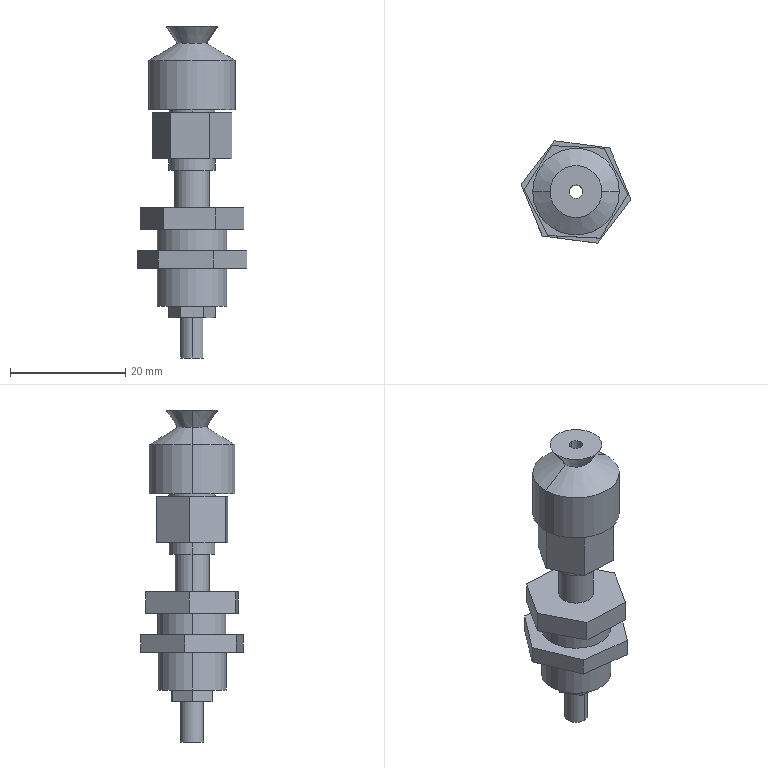Part | STEP file | Suction nozzle SRKN10+SRP9 | 2 solids | 59 faces | box 19.039 x 17.729 x 57.5 mm | volume 5768 mm3 | plane 37 | cylinder 16 | cone 6 | commonest cylinder face diameters 8 x4 12 x4 2.3 x2 4 x2 6 x2 15 x2